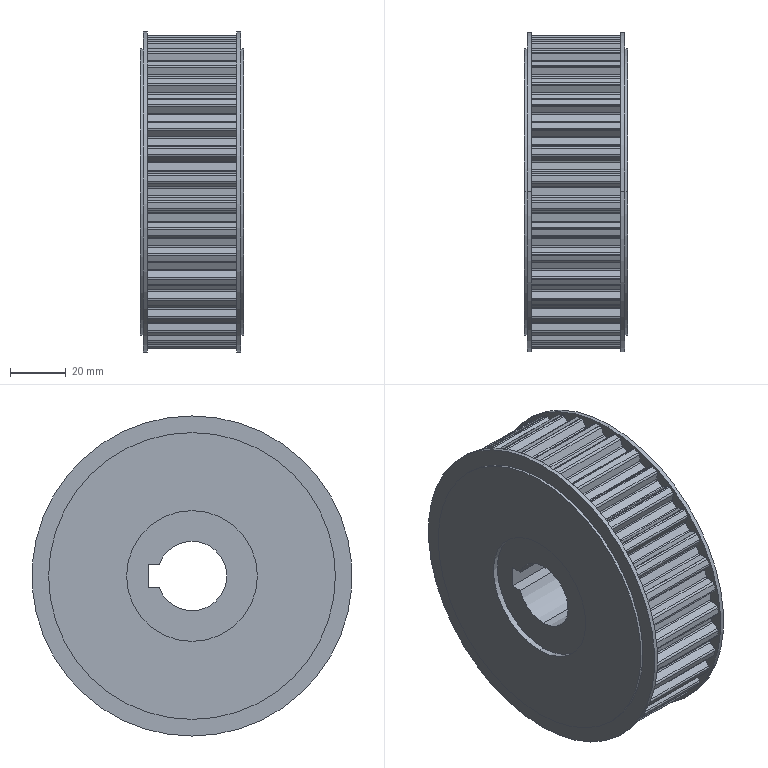Part | SolidWorks | features ICE 6, Fillet 2, HoleWzd 2, MirrorPattern 2, CirPattern 1, Extrusion 1 | 1 solid | 349 faces | box 37 x 115 x 115 mm | volume 322702 mm3 | cylinder 227 | plane 120 | cone 2 | commonest cylinder face diameters 1.2 x86 1.6 x86 112.74 x36 47 x4 103 x4 115 x4